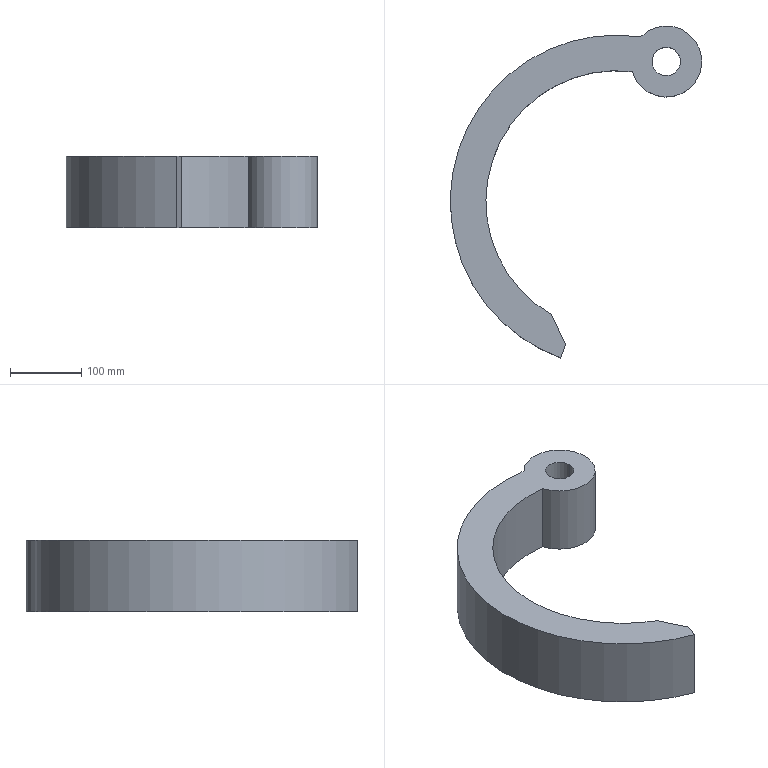Part | SolidWorks | features BossThin 1, Chamfer 1, Cut 1, Extrusion 1 | 1 solid | 9 faces | box 353.552 x 466.663 x 100 mm | volume 3649409 mm3 | cylinder 5 | plane 4 | commonest cylinder face diameters 40 x2 100 x1 367.247 x1 467.247 x1
STEP:
#1=CARTESIAN_POINT('',(-310.,235.,-20.));
#2=VERTEX_POINT('',#1);
#3=CARTESIAN_POINT('',(-270.,235.,-20.));
#4=VERTEX_POINT('',#3);
#5=CARTESIAN_POINT('',(-290.,235.,-20.));
#6=DIRECTION('',(0.,0.,1.));
#7=DIRECTION('',(0.,-1.,0.));
#8=AXIS2_PLACEMENT_3D('',#5,#6,#7);
#9=CIRCLE('',#8,20.);
#10=EDGE_CURVE('',#2,#4,#9,.T.);
#11=ORIENTED_EDGE('',*,*,#10,.F.);
#12=CARTESIAN_POINT('',(-310.,235.,80.));
#13=VERTEX_POINT('',#12);
#14=CARTESIAN_POINT('',(-310.,235.,-61.));
#15=DIRECTION('',(0.,0.,1.));
#16=VECTOR('',#15,1000.);
#17=LINE('',#14,#16);
#18=EDGE_CURVE('',#2,#13,#17,.T.);
#19=ORIENTED_EDGE('',*,*,#18,.T.);
#20=CARTESIAN_POINT('',(-270.,235.,80.));
#21=VERTEX_POINT('',#20);
#22=CARTESIAN_POINT('',(-290.,235.,80.));
#23=DIRECTION('',(0.,0.,1.));
#24=DIRECTION('',(1.,0.,0.));
#25=AXIS2_PLACEMENT_3D('',#22,#23,#24);
#26=CIRCLE('',#25,20.);
#27=EDGE_CURVE('',#13,#21,#26,.T.);
#28=ORIENTED_EDGE('',*,*,#27,.T.);
#29=CARTESIAN_POINT('',(-270.,235.,-61.));
#30=DIRECTION('',(0.,0.,1.));
#31=VECTOR('',#30,1000.);
#32=LINE('',#29,#31);
#33=EDGE_CURVE('',#4,#21,#32,.T.);
#34=ORIENTED_EDGE('',*,*,#33,.F.);
#35=EDGE_LOOP('',(#11,#19,#28,#34));
#36=FACE_OUTER_BOUND('',#35,.T.);
#37=CARTESIAN_POINT('',(-290.,235.,-61.));
#38=DIRECTION('',(0.,0.,1.));
#39=DIRECTION('',(1.,0.,0.));
#40=AXIS2_PLACEMENT_3D('',#37,#38,#39);
#41=CYLINDRICAL_SURFACE('',#40,20.);
#42=ADVANCED_FACE('',(#36),#41,.F.);
#43=CARTESIAN_POINT('',(-337.925,220.746,-20.));
#44=VERTEX_POINT('',#43);
#45=CARTESIAN_POINT('',(-326.09,269.605,-20.));
#46=VERTEX_POINT('',#45);
#47=CARTESIAN_POINT('',(-290.,235.,-20.));
#48=DIRECTION('',(0.,0.,1.));
#49=DIRECTION('',(0.,-1.,0.));
#50=AXIS2_PLACEMENT_3D('',#47,#48,#49);
#51=CIRCLE('',#50,50.);
#52=EDGE_CURVE('',#44,#46,#51,.T.);
#53=ORIENTED_EDGE('',*,*,#52,.T.);
#54=CARTESIAN_POINT('',(-326.09,269.605,80.));
#55=VERTEX_POINT('',#54);
#56=CARTESIAN_POINT('',(-326.09,269.605,30.));
#57=DIRECTION('',(0.,0.,1.));
#58=VECTOR('',#57,1000.);
#59=LINE('',#56,#58);
#60=EDGE_CURVE('',#46,#55,#59,.T.);
#61=ORIENTED_EDGE('',*,*,#60,.T.);
#62=CARTESIAN_POINT('',(-337.925,220.746,80.));
#63=VERTEX_POINT('',#62);
#64=CARTESIAN_POINT('',(-290.,235.,80.));
#65=DIRECTION('',(0.,0.,1.));
#66=DIRECTION('',(0.,-1.,0.));
#67=AXIS2_PLACEMENT_3D('',#64,#65,#66);
#68=CIRCLE('',#67,50.);
#69=EDGE_CURVE('',#63,#55,#68,.T.);
#70=ORIENTED_EDGE('',*,*,#69,.F.);
#71=CARTESIAN_POINT('',(-337.925,220.746,30.));
#72=DIRECTION('',(0.,0.,1.));
#73=VECTOR('',#72,1000.);
#74=LINE('',#71,#73);
#75=EDGE_CURVE('',#44,#63,#74,.T.);
#76=ORIENTED_EDGE('',*,*,#75,.F.);
#77=EDGE_LOOP('',(#53,#61,#70,#76));
#78=FACE_OUTER_BOUND('',#77,.T.);
#79=CARTESIAN_POINT('',(-290.,235.,80.));
#80=DIRECTION('',(0.,0.,-1.));
#81=DIRECTION('',(-1.,0.,0.));
#82=AXIS2_PLACEMENT_3D('',#79,#80,#81);
#83=CYLINDRICAL_SURFACE('',#82,50.);
#84=ADVANCED_FACE('',(#78),#83,.T.);
#85=CARTESIAN_POINT('',(-290.,235.,80.));
#86=DIRECTION('',(0.,0.,1.));
#87=DIRECTION('',(1.,0.,0.));
#88=AXIS2_PLACEMENT_3D('',#85,#86,#87);
#89=CIRCLE('',#88,20.);
#90=EDGE_CURVE('',#21,#13,#89,.T.);
#91=ORIENTED_EDGE('',*,*,#90,.F.);
#92=ORIENTED_EDGE('',*,*,#27,.F.);
#93=EDGE_LOOP('',(#91,#92));
#94=FACE_BOUND('',#93,.T.);
#95=CARTESIAN_POINT('',(-431.534,-162.82,80.));
#96=VERTEX_POINT('',#95);
#97=CARTESIAN_POINT('',(-438.237,-181.663,80.));
#98=VERTEX_POINT('',#97);
#99=CARTESIAN_POINT('',(-421.478,-134.555,80.));
#100=DIRECTION('',(-0.3352,-0.9421,0.));
#101=VECTOR('',#100,1000.);
#102=LINE('',#99,#101);
#103=EDGE_CURVE('',#96,#98,#102,.T.);
#104=ORIENTED_EDGE('',*,*,#103,.F.);
#105=CARTESIAN_POINT('',(-451.556,-120.684,80.));
#106=VERTEX_POINT('',#105);
#107=CARTESIAN_POINT('',(-559.677,106.857,80.));
#108=DIRECTION('',(-0.4292,0.9032,0.));
#109=VECTOR('',#108,1000.);
#110=LINE('',#107,#109);
#111=EDGE_CURVE('',#96,#106,#110,.T.);
#112=ORIENTED_EDGE('',*,*,#111,.T.);
#113=CARTESIAN_POINT('',(-359.929,38.446,80.));
#114=DIRECTION('',(0.,0.,1.));
#115=DIRECTION('',(1.,0.,0.));
#116=AXIS2_PLACEMENT_3D('',#113,#114,#115);
#117=CIRCLE('',#116,183.623);
#118=EDGE_CURVE('',#63,#106,#117,.T.);
#119=ORIENTED_EDGE('',*,*,#118,.F.);
#120=ORIENTED_EDGE('',*,*,#69,.T.);
#121=CARTESIAN_POINT('',(-359.929,38.446,80.));
#122=DIRECTION('',(0.,0.,1.));
#123=DIRECTION('',(1.,0.,0.));
#124=AXIS2_PLACEMENT_3D('',#121,#122,#123);
#125=CIRCLE('',#124,233.623);
#126=EDGE_CURVE('',#55,#98,#125,.T.);
#127=ORIENTED_EDGE('',*,*,#126,.T.);
#128=EDGE_LOOP('',(#104,#112,#119,#120,#127));
#129=FACE_OUTER_BOUND('',#128,.T.);
#130=CARTESIAN_POINT('',(-290.,235.,80.));
#131=DIRECTION('',(0.,0.,1.));
#132=DIRECTION('',(0.,-1.,0.));
#133=AXIS2_PLACEMENT_3D('',#130,#131,#132);
#134=PLANE('',#133);
#135=ADVANCED_FACE('',(#94,#129),#134,.T.);
#136=CARTESIAN_POINT('',(-290.,235.,-20.));
#137=DIRECTION('',(0.,0.,1.));
#138=DIRECTION('',(0.,-1.,0.));
#139=AXIS2_PLACEMENT_3D('',#136,#137,#138);
#140=CIRCLE('',#139,20.);
#141=EDGE_CURVE('',#4,#2,#140,.T.);
#142=ORIENTED_EDGE('',*,*,#141,.T.);
#143=ORIENTED_EDGE('',*,*,#10,.T.);
#144=EDGE_LOOP('',(#142,#143));
#145=FACE_BOUND('',#144,.T.);
#146=CARTESIAN_POINT('',(-451.556,-120.684,-20.));
#147=VERTEX_POINT('',#146);
#148=CARTESIAN_POINT('',(-359.929,38.446,-20.));
#149=DIRECTION('',(0.,0.,1.));
#150=DIRECTION('',(1.,0.,0.));
#151=AXIS2_PLACEMENT_3D('',#148,#149,#150);
#152=CIRCLE('',#151,183.623);
#153=EDGE_CURVE('',#44,#147,#152,.T.);
#154=ORIENTED_EDGE('',*,*,#153,.T.);
#155=CARTESIAN_POINT('',(-431.534,-162.82,-20.));
#156=VERTEX_POINT('',#155);
#157=CARTESIAN_POINT('',(-431.534,-162.82,-20.));
#158=DIRECTION('',(0.4292,-0.9032,0.));
#159=VECTOR('',#158,1000.);
#160=LINE('',#157,#159);
#161=EDGE_CURVE('',#147,#156,#160,.T.);
#162=ORIENTED_EDGE('',*,*,#161,.T.);
#163=CARTESIAN_POINT('',(-438.237,-181.663,-20.));
#164=VERTEX_POINT('',#163);
#165=CARTESIAN_POINT('',(-421.478,-134.555,-20.));
#166=DIRECTION('',(-0.3352,-0.9421,0.));
#167=VECTOR('',#166,1000.);
#168=LINE('',#165,#167);
#169=EDGE_CURVE('',#156,#164,#168,.T.);
#170=ORIENTED_EDGE('',*,*,#169,.T.);
#171=CARTESIAN_POINT('',(-359.929,38.446,-20.));
#172=DIRECTION('',(0.,0.,1.));
#173=DIRECTION('',(1.,0.,0.));
#174=AXIS2_PLACEMENT_3D('',#171,#172,#173);
#175=CIRCLE('',#174,233.623);
#176=EDGE_CURVE('',#46,#164,#175,.T.);
#177=ORIENTED_EDGE('',*,*,#176,.F.);
#178=ORIENTED_EDGE('',*,*,#52,.F.);
#179=EDGE_LOOP('',(#154,#162,#170,#177,#178));
#180=FACE_OUTER_BOUND('',#179,.T.);
#181=CARTESIAN_POINT('',(-290.,235.,-20.));
#182=DIRECTION('',(0.,0.,1.));
#183=DIRECTION('',(0.,-1.,0.));
#184=AXIS2_PLACEMENT_3D('',#181,#182,#183);
#185=PLANE('',#184);
#186=ADVANCED_FACE('',(#145,#180),#185,.F.);
#187=ORIENTED_EDGE('',*,*,#60,.F.);
#188=ORIENTED_EDGE('',*,*,#176,.T.);
#189=CARTESIAN_POINT('',(-438.237,-181.663,-20.));
#190=DIRECTION('',(0.,0.,1.));
#191=VECTOR('',#190,1000.);
#192=LINE('',#189,#191);
#193=EDGE_CURVE('',#164,#98,#192,.T.);
#194=ORIENTED_EDGE('',*,*,#193,.T.);
#195=ORIENTED_EDGE('',*,*,#126,.F.);
#196=EDGE_LOOP('',(#187,#188,#194,#195));
#197=FACE_OUTER_BOUND('',#196,.T.);
#198=CARTESIAN_POINT('',(-359.929,38.446,-20.));
#199=DIRECTION('',(0.,0.,1.));
#200=DIRECTION('',(1.,0.,0.));
#201=AXIS2_PLACEMENT_3D('',#198,#199,#200);
#202=CYLINDRICAL_SURFACE('',#201,233.623);
#203=ADVANCED_FACE('',(#197),#202,.T.);
#204=ORIENTED_EDGE('',*,*,#118,.T.);
#205=CARTESIAN_POINT('',(-451.556,-120.684,-20.));
#206=DIRECTION('',(0.,0.,-1.));
#207=VECTOR('',#206,1000.);
#208=LINE('',#205,#207);
#209=EDGE_CURVE('',#106,#147,#208,.T.);
#210=ORIENTED_EDGE('',*,*,#209,.T.);
#211=ORIENTED_EDGE('',*,*,#153,.F.);
#212=ORIENTED_EDGE('',*,*,#75,.T.);
#213=EDGE_LOOP('',(#204,#210,#211,#212));
#214=FACE_OUTER_BOUND('',#213,.T.);
#215=CARTESIAN_POINT('',(-359.929,38.446,-20.));
#216=DIRECTION('',(0.,0.,1.));
#217=DIRECTION('',(1.,0.,0.));
#218=AXIS2_PLACEMENT_3D('',#215,#216,#217);
#219=CYLINDRICAL_SURFACE('',#218,183.623);
#220=ADVANCED_FACE('',(#214),#219,.F.);
#221=ORIENTED_EDGE('',*,*,#169,.F.);
#222=CARTESIAN_POINT('',(-431.534,-162.82,-20.));
#223=DIRECTION('',(0.,0.,1.));
#224=VECTOR('',#223,1000.);
#225=LINE('',#222,#224);
#226=EDGE_CURVE('',#156,#96,#225,.T.);
#227=ORIENTED_EDGE('',*,*,#226,.T.);
#228=ORIENTED_EDGE('',*,*,#103,.T.);
#229=ORIENTED_EDGE('',*,*,#193,.F.);
#230=EDGE_LOOP('',(#221,#227,#228,#229));
#231=FACE_OUTER_BOUND('',#230,.T.);
#232=CARTESIAN_POINT('',(-421.478,-134.555,-20.));
#233=DIRECTION('',(-0.9421,0.3352,0.));
#234=DIRECTION('',(-0.3352,-0.9421,0.));
#235=AXIS2_PLACEMENT_3D('',#232,#233,#234);
#236=PLANE('',#235);
#237=ADVANCED_FACE('',(#231),#236,.F.);
#238=ORIENTED_EDGE('',*,*,#161,.F.);
#239=ORIENTED_EDGE('',*,*,#209,.F.);
#240=ORIENTED_EDGE('',*,*,#111,.F.);
#241=ORIENTED_EDGE('',*,*,#226,.F.);
#242=EDGE_LOOP('',(#238,#239,#240,#241));
#243=FACE_OUTER_BOUND('',#242,.T.);
#244=CARTESIAN_POINT('',(-431.534,-162.82,-20.));
#245=DIRECTION('',(-0.9032,-0.4292,0.));
#246=DIRECTION('',(0.,0.,1.));
#247=AXIS2_PLACEMENT_3D('',#244,#245,#246);
#248=PLANE('',#247);
#249=ADVANCED_FACE('',(#243),#248,.F.);
#250=ORIENTED_EDGE('',*,*,#18,.F.);
#251=ORIENTED_EDGE('',*,*,#141,.F.);
#252=ORIENTED_EDGE('',*,*,#33,.T.);
#253=ORIENTED_EDGE('',*,*,#90,.T.);
#254=EDGE_LOOP('',(#250,#251,#252,#253));
#255=FACE_OUTER_BOUND('',#254,.T.);
#256=CARTESIAN_POINT('',(-290.,235.,-61.));
#257=DIRECTION('',(0.,0.,1.));
#258=DIRECTION('',(1.,0.,0.));
#259=AXIS2_PLACEMENT_3D('',#256,#257,#258);
#260=CYLINDRICAL_SURFACE('',#259,20.);
#261=ADVANCED_FACE('',(#255),#260,.F.);
#262=CLOSED_SHELL('',(#42,#84,#135,#186,#203,#220,#237,#249,#261));
#263=MANIFOLD_SOLID_BREP('',#262);
#264=CARTESIAN_POINT('',(0.,0.,0.));
#265=DIRECTION('',(0.,0.,1.));
#266=DIRECTION('',(1.,0.,0.));
#267=AXIS2_PLACEMENT_3D('',#264,#265,#266);
#268=(LENGTH_UNIT()NAMED_UNIT(*)SI_UNIT(.MILLI.,.METRE.));
#269=UNCERTAINTY_MEASURE_WITH_UNIT(LENGTH_MEASURE(0.00001),#268,'','');
#270=(NAMED_UNIT(*)PLANE_ANGLE_UNIT()SI_UNIT($,.RADIAN.));
#271=(NAMED_UNIT(*)SI_UNIT($,.STERADIAN.)SOLID_ANGLE_UNIT());
#272=(GEOMETRIC_REPRESENTATION_CONTEXT(3)GLOBAL_UNCERTAINTY_ASSIGNED_CONTEXT((#269))GLOBAL_UNIT_ASSIGNED_CONTEXT((#268,#270,#271))REPRESENTATION_CONTEXT('',''));
#273=ADVANCED_BREP_SHAPE_REPRESENTATION('',(#263,#267),#272);